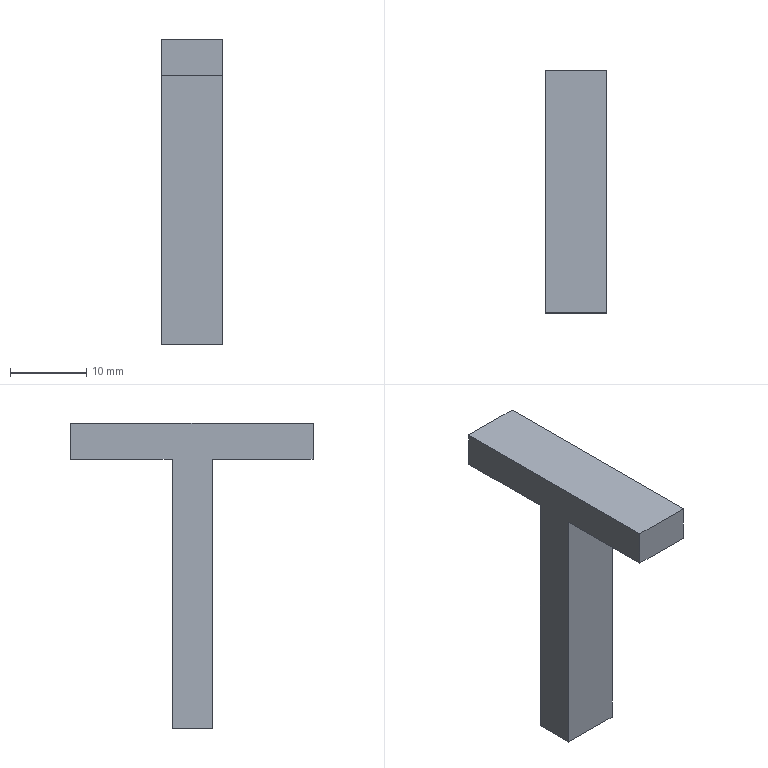Part | NX | features solid 2 | 1 solid | 10 faces | box 8 x 31.701 x 40 mm | volume 2690 mm3 | plane 10
STEP:
#1=CARTESIAN_POINT('',(2258.,587.155,-669.685));
#2=VERTEX_POINT('',#1);
#3=CARTESIAN_POINT('',(2258.,592.446,-669.685));
#4=VERTEX_POINT('',#3);
#5=CARTESIAN_POINT('',(2258.,592.446,-669.685));
#6=DIRECTION('',(0.,1.,0.));
#7=VECTOR('',#6,1000.);
#8=LINE('',#5,#7);
#9=EDGE_CURVE('',#2,#4,#8,.T.);
#10=ORIENTED_EDGE('',*,*,#9,.F.);
#11=CARTESIAN_POINT('',(2250.,587.155,-669.685));
#12=VERTEX_POINT('',#11);
#13=CARTESIAN_POINT('',(2250.,587.155,-669.685));
#14=DIRECTION('',(1.,0.,0.));
#15=VECTOR('',#14,1000.);
#16=LINE('',#13,#15);
#17=EDGE_CURVE('',#12,#2,#16,.T.);
#18=ORIENTED_EDGE('',*,*,#17,.F.);
#19=CARTESIAN_POINT('',(2250.,592.446,-669.685));
#20=VERTEX_POINT('',#19);
#21=CARTESIAN_POINT('',(2250.,592.446,-669.685));
#22=CARTESIAN_POINT('',(2250.,590.682,-669.685));
#23=CARTESIAN_POINT('',(2250.,588.919,-669.685));
#24=CARTESIAN_POINT('',(2250.,587.155,-669.685));
#25=B_SPLINE_CURVE_WITH_KNOTS('',3,(#21,#22,#23,#24),.UNSPECIFIED.,.F.,.F.,(4,4),(0.,0.03689),.PIECEWISE_BEZIER_KNOTS.);
#26=EDGE_CURVE('',#20,#12,#25,.T.);
#27=ORIENTED_EDGE('',*,*,#26,.F.);
#28=CARTESIAN_POINT('',(2250.,592.446,-669.685));
#29=DIRECTION('',(1.,0.,0.));
#30=VECTOR('',#29,1000.);
#31=LINE('',#28,#30);
#32=EDGE_CURVE('',#20,#4,#31,.T.);
#33=ORIENTED_EDGE('',*,*,#32,.T.);
#34=EDGE_LOOP('',(#10,#18,#27,#33));
#35=FACE_BOUND('',#34,.T.);
#36=CARTESIAN_POINT('',(2250.,592.446,-669.685));
#37=DIRECTION('',(0.,0.,-1.));
#38=DIRECTION('',(1.,0.,0.));
#39=AXIS2_PLACEMENT_3D('',#36,#37,#38);
#40=PLANE('',#39);
#41=ADVANCED_FACE('',(#35),#40,.T.);
#42=CARTESIAN_POINT('',(2258.,587.155,-634.403));
#43=VERTEX_POINT('',#42);
#44=CARTESIAN_POINT('',(2258.,587.155,-669.685));
#45=DIRECTION('',(0.,0.,-1.));
#46=VECTOR('',#45,1000.);
#47=LINE('',#44,#46);
#48=EDGE_CURVE('',#43,#2,#47,.T.);
#49=ORIENTED_EDGE('',*,*,#48,.F.);
#50=CARTESIAN_POINT('',(2250.,587.155,-634.403));
#51=VERTEX_POINT('',#50);
#52=CARTESIAN_POINT('',(2250.,587.155,-634.403));
#53=DIRECTION('',(1.,0.,0.));
#54=VECTOR('',#53,1000.);
#55=LINE('',#52,#54);
#56=EDGE_CURVE('',#51,#43,#55,.T.);
#57=ORIENTED_EDGE('',*,*,#56,.F.);
#58=CARTESIAN_POINT('',(2250.,587.155,-669.685));
#59=CARTESIAN_POINT('',(2250.,587.155,-657.924));
#60=CARTESIAN_POINT('',(2250.,587.155,-646.164));
#61=CARTESIAN_POINT('',(2250.,587.155,-634.403));
#62=B_SPLINE_CURVE_WITH_KNOTS('',3,(#58,#59,#60,#61),.UNSPECIFIED.,.F.,.F.,(4,4),(0.03689,0.2829),.PIECEWISE_BEZIER_KNOTS.);
#63=EDGE_CURVE('',#12,#51,#62,.T.);
#64=ORIENTED_EDGE('',*,*,#63,.F.);
#65=ORIENTED_EDGE('',*,*,#17,.T.);
#66=EDGE_LOOP('',(#49,#57,#64,#65));
#67=FACE_BOUND('',#66,.T.);
#68=CARTESIAN_POINT('',(2250.,587.155,-669.685));
#69=DIRECTION('',(0.,-1.,0.));
#70=DIRECTION('',(-1.,0.,0.));
#71=AXIS2_PLACEMENT_3D('',#68,#69,#70);
#72=PLANE('',#71);
#73=ADVANCED_FACE('',(#67),#72,.T.);
#74=CARTESIAN_POINT('',(2258.,573.975,-634.403));
#75=VERTEX_POINT('',#74);
#76=CARTESIAN_POINT('',(2258.,587.155,-634.403));
#77=DIRECTION('',(0.,1.,0.));
#78=VECTOR('',#77,1000.);
#79=LINE('',#76,#78);
#80=EDGE_CURVE('',#75,#43,#79,.T.);
#81=ORIENTED_EDGE('',*,*,#80,.F.);
#82=CARTESIAN_POINT('',(2250.,573.975,-634.403));
#83=VERTEX_POINT('',#82);
#84=CARTESIAN_POINT('',(2250.,573.975,-634.403));
#85=DIRECTION('',(1.,0.,0.));
#86=VECTOR('',#85,1000.);
#87=LINE('',#84,#86);
#88=EDGE_CURVE('',#83,#75,#87,.T.);
#89=ORIENTED_EDGE('',*,*,#88,.F.);
#90=CARTESIAN_POINT('',(2250.,587.155,-634.403));
#91=CARTESIAN_POINT('',(2250.,582.762,-634.403));
#92=CARTESIAN_POINT('',(2250.,578.369,-634.403));
#93=CARTESIAN_POINT('',(2250.,573.975,-634.403));
#94=B_SPLINE_CURVE_WITH_KNOTS('',3,(#90,#91,#92,#93),.UNSPECIFIED.,.F.,.F.,(4,4),(0.2829,0.3748),.PIECEWISE_BEZIER_KNOTS.);
#95=EDGE_CURVE('',#51,#83,#94,.T.);
#96=ORIENTED_EDGE('',*,*,#95,.F.);
#97=ORIENTED_EDGE('',*,*,#56,.T.);
#98=EDGE_LOOP('',(#81,#89,#96,#97));
#99=FACE_BOUND('',#98,.T.);
#100=CARTESIAN_POINT('',(2250.,587.155,-634.403));
#101=DIRECTION('',(0.,0.,-1.));
#102=DIRECTION('',(1.,0.,0.));
#103=AXIS2_PLACEMENT_3D('',#100,#101,#102);
#104=PLANE('',#103);
#105=ADVANCED_FACE('',(#99),#104,.T.);
#106=CARTESIAN_POINT('',(2258.,573.975,-629.685));
#107=VERTEX_POINT('',#106);
#108=CARTESIAN_POINT('',(2258.,573.975,-634.403));
#109=DIRECTION('',(0.,0.,-1.));
#110=VECTOR('',#109,1000.);
#111=LINE('',#108,#110);
#112=EDGE_CURVE('',#107,#75,#111,.T.);
#113=ORIENTED_EDGE('',*,*,#112,.F.);
#114=CARTESIAN_POINT('',(2250.,573.975,-629.685));
#115=VERTEX_POINT('',#114);
#116=CARTESIAN_POINT('',(2250.,573.975,-629.685));
#117=DIRECTION('',(1.,0.,0.));
#118=VECTOR('',#117,1000.);
#119=LINE('',#116,#118);
#120=EDGE_CURVE('',#115,#107,#119,.T.);
#121=ORIENTED_EDGE('',*,*,#120,.F.);
#122=CARTESIAN_POINT('',(2250.,573.975,-634.403));
#123=CARTESIAN_POINT('',(2250.,573.975,-632.83));
#124=CARTESIAN_POINT('',(2250.,573.975,-631.258));
#125=CARTESIAN_POINT('',(2250.,573.975,-629.685));
#126=B_SPLINE_CURVE_WITH_KNOTS('',3,(#122,#123,#124,#125),.UNSPECIFIED.,.F.,.F.,(4,4),(0.3748,0.4077),.PIECEWISE_BEZIER_KNOTS.);
#127=EDGE_CURVE('',#83,#115,#126,.T.);
#128=ORIENTED_EDGE('',*,*,#127,.F.);
#129=ORIENTED_EDGE('',*,*,#88,.T.);
#130=EDGE_LOOP('',(#113,#121,#128,#129));
#131=FACE_BOUND('',#130,.T.);
#132=CARTESIAN_POINT('',(2250.,573.975,-634.403));
#133=DIRECTION('',(0.,-1.,0.));
#134=DIRECTION('',(-1.,0.,0.));
#135=AXIS2_PLACEMENT_3D('',#132,#133,#134);
#136=PLANE('',#135);
#137=ADVANCED_FACE('',(#131),#136,.T.);
#138=CARTESIAN_POINT('',(2258.,605.677,-629.685));
#139=VERTEX_POINT('',#138);
#140=CARTESIAN_POINT('',(2258.,573.975,-629.685));
#141=DIRECTION('',(0.,-1.,0.));
#142=VECTOR('',#141,1000.);
#143=LINE('',#140,#142);
#144=EDGE_CURVE('',#139,#107,#143,.T.);
#145=ORIENTED_EDGE('',*,*,#144,.F.);
#146=CARTESIAN_POINT('',(2250.,605.677,-629.685));
#147=VERTEX_POINT('',#146);
#148=CARTESIAN_POINT('',(2250.,605.677,-629.685));
#149=DIRECTION('',(1.,0.,0.));
#150=VECTOR('',#149,1000.);
#151=LINE('',#148,#150);
#152=EDGE_CURVE('',#147,#139,#151,.T.);
#153=ORIENTED_EDGE('',*,*,#152,.F.);
#154=CARTESIAN_POINT('',(2250.,573.975,-629.685));
#155=CARTESIAN_POINT('',(2250.,584.542,-629.685));
#156=CARTESIAN_POINT('',(2250.,595.11,-629.685));
#157=CARTESIAN_POINT('',(2250.,605.677,-629.685));
#158=B_SPLINE_CURVE_WITH_KNOTS('',3,(#154,#155,#156,#157),.UNSPECIFIED.,.F.,.F.,(4,4),(0.4077,0.6288),.PIECEWISE_BEZIER_KNOTS.);
#159=EDGE_CURVE('',#115,#147,#158,.T.);
#160=ORIENTED_EDGE('',*,*,#159,.F.);
#161=ORIENTED_EDGE('',*,*,#120,.T.);
#162=EDGE_LOOP('',(#145,#153,#160,#161));
#163=FACE_BOUND('',#162,.T.);
#164=CARTESIAN_POINT('',(2250.,573.975,-629.685));
#165=DIRECTION('',(0.,0.,1.));
#166=DIRECTION('',(-1.,0.,0.));
#167=AXIS2_PLACEMENT_3D('',#164,#165,#166);
#168=PLANE('',#167);
#169=ADVANCED_FACE('',(#163),#168,.T.);
#170=CARTESIAN_POINT('',(2258.,605.677,-634.403));
#171=VERTEX_POINT('',#170);
#172=CARTESIAN_POINT('',(2258.,605.677,-629.685));
#173=DIRECTION('',(0.,0.,1.));
#174=VECTOR('',#173,1000.);
#175=LINE('',#172,#174);
#176=EDGE_CURVE('',#171,#139,#175,.T.);
#177=ORIENTED_EDGE('',*,*,#176,.F.);
#178=CARTESIAN_POINT('',(2250.,605.677,-634.403));
#179=VERTEX_POINT('',#178);
#180=CARTESIAN_POINT('',(2250.,605.677,-634.403));
#181=DIRECTION('',(1.,0.,0.));
#182=VECTOR('',#181,1000.);
#183=LINE('',#180,#182);
#184=EDGE_CURVE('',#179,#171,#183,.T.);
#185=ORIENTED_EDGE('',*,*,#184,.F.);
#186=CARTESIAN_POINT('',(2250.,605.677,-629.685));
#187=CARTESIAN_POINT('',(2250.,605.677,-631.258));
#188=CARTESIAN_POINT('',(2250.,605.677,-632.83));
#189=CARTESIAN_POINT('',(2250.,605.677,-634.403));
#190=B_SPLINE_CURVE_WITH_KNOTS('',3,(#186,#187,#188,#189),.UNSPECIFIED.,.F.,.F.,(4,4),(0.6288,0.6617),.PIECEWISE_BEZIER_KNOTS.);
#191=EDGE_CURVE('',#147,#179,#190,.T.);
#192=ORIENTED_EDGE('',*,*,#191,.F.);
#193=ORIENTED_EDGE('',*,*,#152,.T.);
#194=EDGE_LOOP('',(#177,#185,#192,#193));
#195=FACE_BOUND('',#194,.T.);
#196=CARTESIAN_POINT('',(2250.,605.677,-629.685));
#197=DIRECTION('',(0.,1.,0.));
#198=DIRECTION('',(1.,0.,0.));
#199=AXIS2_PLACEMENT_3D('',#196,#197,#198);
#200=PLANE('',#199);
#201=ADVANCED_FACE('',(#195),#200,.T.);
#202=CARTESIAN_POINT('',(2258.,592.446,-634.403));
#203=VERTEX_POINT('',#202);
#204=CARTESIAN_POINT('',(2258.,605.677,-634.403));
#205=DIRECTION('',(0.,1.,0.));
#206=VECTOR('',#205,1000.);
#207=LINE('',#204,#206);
#208=EDGE_CURVE('',#203,#171,#207,.T.);
#209=ORIENTED_EDGE('',*,*,#208,.F.);
#210=CARTESIAN_POINT('',(2250.,592.446,-634.403));
#211=VERTEX_POINT('',#210);
#212=CARTESIAN_POINT('',(2250.,592.446,-634.403));
#213=DIRECTION('',(1.,0.,0.));
#214=VECTOR('',#213,1000.);
#215=LINE('',#212,#214);
#216=EDGE_CURVE('',#211,#203,#215,.T.);
#217=ORIENTED_EDGE('',*,*,#216,.F.);
#218=CARTESIAN_POINT('',(2250.,605.677,-634.403));
#219=CARTESIAN_POINT('',(2250.,601.266,-634.403));
#220=CARTESIAN_POINT('',(2250.,596.856,-634.403));
#221=CARTESIAN_POINT('',(2250.,592.446,-634.403));
#222=B_SPLINE_CURVE_WITH_KNOTS('',3,(#218,#219,#220,#221),.UNSPECIFIED.,.F.,.F.,(4,4),(0.6617,0.754),.PIECEWISE_BEZIER_KNOTS.);
#223=EDGE_CURVE('',#179,#211,#222,.T.);
#224=ORIENTED_EDGE('',*,*,#223,.F.);
#225=ORIENTED_EDGE('',*,*,#184,.T.);
#226=EDGE_LOOP('',(#209,#217,#224,#225));
#227=FACE_BOUND('',#226,.T.);
#228=CARTESIAN_POINT('',(2250.,605.677,-634.403));
#229=DIRECTION('',(0.,0.,-1.));
#230=DIRECTION('',(1.,0.,0.));
#231=AXIS2_PLACEMENT_3D('',#228,#229,#230);
#232=PLANE('',#231);
#233=ADVANCED_FACE('',(#227),#232,.T.);
#234=CARTESIAN_POINT('',(2258.,592.446,-634.403));
#235=DIRECTION('',(0.,0.,1.));
#236=VECTOR('',#235,1000.);
#237=LINE('',#234,#236);
#238=EDGE_CURVE('',#4,#203,#237,.T.);
#239=ORIENTED_EDGE('',*,*,#238,.F.);
#240=ORIENTED_EDGE('',*,*,#32,.F.);
#241=CARTESIAN_POINT('',(2250.,592.446,-634.403));
#242=CARTESIAN_POINT('',(2250.,592.446,-646.164));
#243=CARTESIAN_POINT('',(2250.,592.446,-657.924));
#244=CARTESIAN_POINT('',(2250.,592.446,-669.685));
#245=B_SPLINE_CURVE_WITH_KNOTS('',3,(#241,#242,#243,#244),.UNSPECIFIED.,.F.,.F.,(4,4),(0.754,1.),.PIECEWISE_BEZIER_KNOTS.);
#246=EDGE_CURVE('',#211,#20,#245,.T.);
#247=ORIENTED_EDGE('',*,*,#246,.F.);
#248=ORIENTED_EDGE('',*,*,#216,.T.);
#249=EDGE_LOOP('',(#239,#240,#247,#248));
#250=FACE_BOUND('',#249,.T.);
#251=CARTESIAN_POINT('',(2250.,592.446,-634.403));
#252=DIRECTION('',(0.,1.,0.));
#253=DIRECTION('',(1.,0.,0.));
#254=AXIS2_PLACEMENT_3D('',#251,#252,#253);
#255=PLANE('',#254);
#256=ADVANCED_FACE('',(#250),#255,.T.);
#257=ORIENTED_EDGE('',*,*,#26,.T.);
#258=ORIENTED_EDGE('',*,*,#63,.T.);
#259=ORIENTED_EDGE('',*,*,#95,.T.);
#260=ORIENTED_EDGE('',*,*,#127,.T.);
#261=ORIENTED_EDGE('',*,*,#159,.T.);
#262=ORIENTED_EDGE('',*,*,#191,.T.);
#263=ORIENTED_EDGE('',*,*,#223,.T.);
#264=ORIENTED_EDGE('',*,*,#246,.T.);
#265=EDGE_LOOP('',(#257,#258,#259,#260,#261,#262,#263,#264));
#266=FACE_BOUND('',#265,.T.);
#267=CARTESIAN_POINT('',(2250.,589.8,-669.685));
#268=DIRECTION('',(-1.,0.,0.));
#269=DIRECTION('',(0.,1.,0.));
#270=AXIS2_PLACEMENT_3D('',#267,#268,#269);
#271=PLANE('',#270);
#272=ADVANCED_FACE('',(#266),#271,.T.);
#273=ORIENTED_EDGE('',*,*,#48,.T.);
#274=ORIENTED_EDGE('',*,*,#9,.T.);
#275=ORIENTED_EDGE('',*,*,#238,.T.);
#276=ORIENTED_EDGE('',*,*,#208,.T.);
#277=ORIENTED_EDGE('',*,*,#176,.T.);
#278=ORIENTED_EDGE('',*,*,#144,.T.);
#279=ORIENTED_EDGE('',*,*,#112,.T.);
#280=ORIENTED_EDGE('',*,*,#80,.T.);
#281=EDGE_LOOP('',(#273,#274,#275,#276,#277,#278,#279,#280));
#282=FACE_BOUND('',#281,.T.);
#283=CARTESIAN_POINT('',(2258.,543.819,-626.247));
#284=DIRECTION('',(-1.,0.,0.));
#285=DIRECTION('',(0.,0.,-1.));
#286=AXIS2_PLACEMENT_3D('',#283,#284,#285);
#287=PLANE('',#286);
#288=ADVANCED_FACE('',(#282),#287,.F.);
#289=CLOSED_SHELL('',(#41,#73,#105,#137,#169,#201,#233,#256,#272,#288));
#290=MANIFOLD_SOLID_BREP('',#289);
#291=(LENGTH_UNIT()NAMED_UNIT(*)SI_UNIT(.MILLI.,.METRE.));
#292=UNCERTAINTY_MEASURE_WITH_UNIT(LENGTH_MEASURE(0.00001),#291,'','');
#293=(NAMED_UNIT(*)PLANE_ANGLE_UNIT()SI_UNIT($,.RADIAN.));
#294=(NAMED_UNIT(*)SI_UNIT($,.STERADIAN.)SOLID_ANGLE_UNIT());
#295=(GEOMETRIC_REPRESENTATION_CONTEXT(3)GLOBAL_UNCERTAINTY_ASSIGNED_CONTEXT((#292))GLOBAL_UNIT_ASSIGNED_CONTEXT((#291,#293,#294))REPRESENTATION_CONTEXT('',''));
#296=ADVANCED_BREP_SHAPE_REPRESENTATION('',(#290),#295);